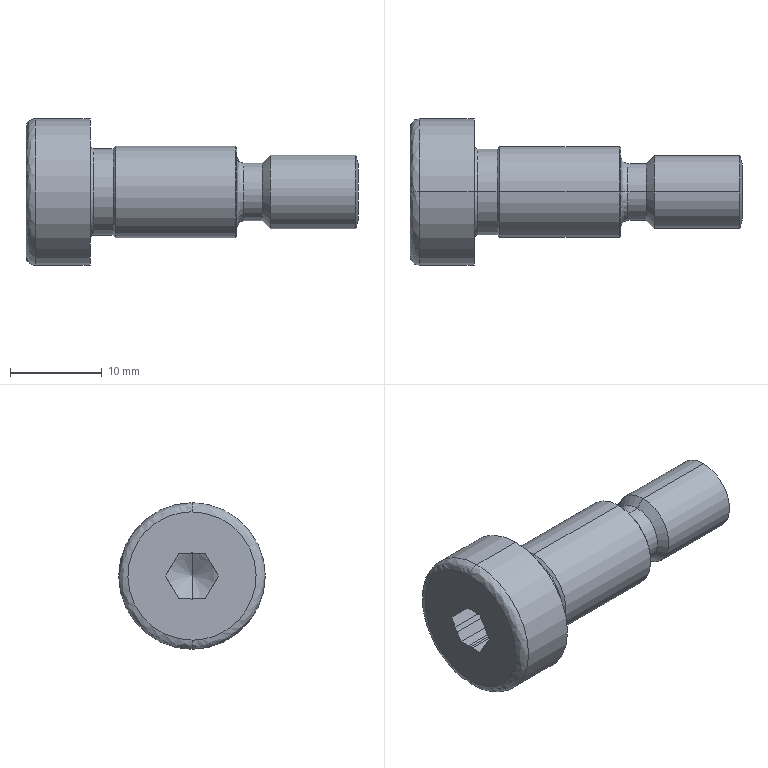Part | STEP file | ANSI B18.3.3M - M8x1,25 x 29,25 | 1 solid | 43 faces | box 36.25 x 16 x 16 mm | volume 3128 mm3 | cylinder 17 | cone 10 | plane 10 | spline 6 | commonest cylinder face diameters 5.033 x7 6.25 x2 8 x2 9.42 x2 10 x2 16 x2